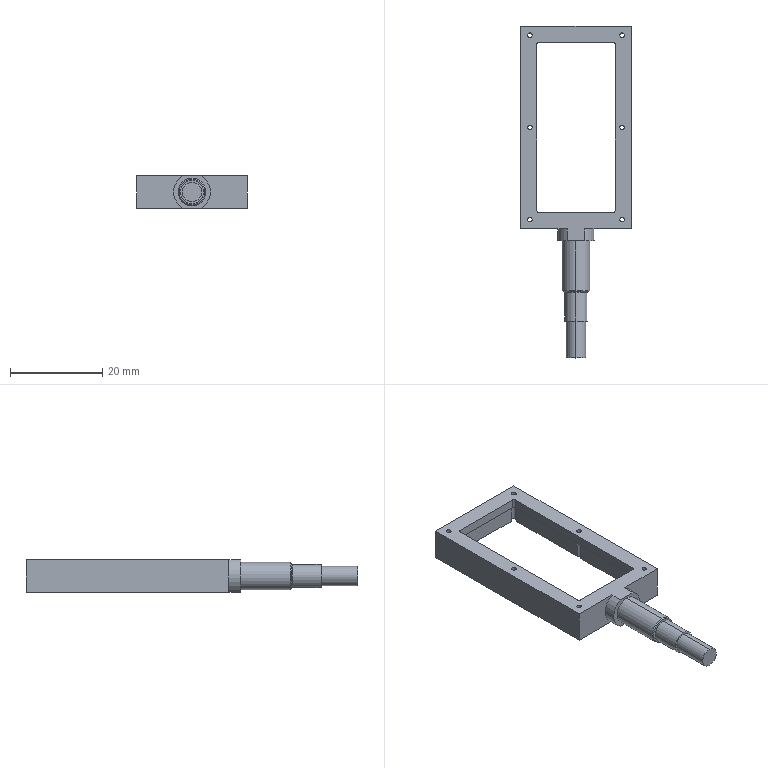NC program | NX | posted with a generic post | part box 24 x 72 x 7 mm
Whole program:
N10 G17 G21 G94 G90
(FLOOR_WALL_COPY , TOOL : D10)
N12 T10 M6
N14 G54
N16 G17 G0 G90 X22. Y11.482 S9500 M3
N18 G43 Z37. H10
N20 Z18.505
N22 G94 G1 Z15.505 F1000.
N24 Y3.482
N26 X0. F2500.
N28 Y-3.482
N30 X44.
N32 Y3.482
N34 X22.
N36 Y11.482
N38 Z18.505
N40 G0 Z37.
N42 Y12.873
N44 Z18.011
N46 G1 Z15.011 F1000.
N48 Y-0.373
N50 X39.5 F2500.
N52 Y0.373
N54 X4.5
N56 Y-0.373
N58 X22.
N60 Y-4.873
N62 X44.
N64 Y4.873
N66 X0.
N68 Y-4.873
N70 X22.
N72 Y-12.873
N74 Z18.011
N76 G0 Z37.
N78 Y-13.907
N80 Z17.516
N82 G1 Z14.516 F1000.
N84 Y-0.907
N86 X39. F2500.
N88 Y0.907
N90 X5.
N92 Y-0.907
N94 X22.
N96 Y-5.907
N98 X44.
N100 Y5.907
N102 X0.
N104 Y-5.907
N106 X22.
N108 Y-13.907
N110 Z17.516
N112 G0 Z37.
N114 Y-14.748
N116 Z17.022
N118 G1 Z14.022 F1000.
N120 Y-1.748
N122 X39. F2500.
N124 Y1.748
N126 X5.
N128 Y-1.748
N130 X22.
N132 Y-6.748
N134 X44.
N136 Y6.748
N138 X0.
N140 Y-6.748
N142 X22.
N144 Y-14.748
N146 Z17.022
N148 G0 Z37.
N150 Y-15.463
N152 Z16.528
N154 G1 Z13.528 F1000.
N156 Y-2.463
N158 X39. F2500.
N160 Y2.463
N162 X5.
N164 Y-2.463
N166 X22.
N168 Y-7.463
N170 X44.
N172 Y7.463
N174 X0.
N176 Y-7.463
N178 X22.
N180 Y-15.463
N182 Z16.528
N184 G0 Z37.
N186 Y-16.085
N188 Z16.033
N190 G1 Z13.033 F1000.
N192 Y-3.085
N194 X39. F2500.
N196 Y3.085
N198 X5.
N200 Y-3.085
N202 X22.
N204 Y-8.085
N206 X44.
N208 Y8.085
N210 X0.
N212 Y-8.085
N214 X22.
N216 Y-16.085
N218 Z16.033
N220 G0 Z37.
N222 Y-16.634
N224 Z15.539
N226 G1 Z12.539 F1000.
N228 Y-3.634
N230 X39. F2500.
N232 Y3.634
N234 X5.
N236 Y-3.634
N238 X22.
N240 Y-8.634
N242 X44.
N244 Y8.634
N246 X0.
N248 Y-8.634
N250 X22.
N252 Y-16.634
N254 Z15.539
N256 G0 Z37.
N258 Y-17.124
N260 Z15.044
N262 G1 Z12.044 F1000.
N264 Y-4.124
N266 X39. F2500.
N268 Y4.124
N270 X5.
N272 Y-4.124
N274 X22.
N276 Y-9.124
N278 X44.
N280 Y9.124
N282 X0.
N284 Y-9.124
N286 X22.
N288 Y-17.124
N290 Z15.044
N292 G0 Z37.
N294 X9.915 Y0.063
N296 Z15.044
N298 G1 X9.5 Z14.933 F1000.
N300 Y-0.063 Z14.899
N302 X22. Z11.55
N304 X34.5 F2500.
N306 Y0.063
N308 X9.5
N310 Y-0.063
N312 X22.
N314 Y-4.563
N316 X39.
N318 Y4.563
N320 X5.
N322 Y-4.563
N324 X22.
N326 Y-9.563
N328 X44.
N330 Y9.563
N332 X0.
N334 Y-9.563
N336 X22.
N338 Y-17.563
N340 Z14.55
N342 G0 Z37.
N344 X9.5 Y0.083
N346 Z14.55
N348 G1 Y-0.458 Z14.405 F1000.
N350 X22. Z11.055
N352 X34.5 F2500.
N354 Y0.458
N356 X9.5
N358 Y-0.458
N360 X22.
N362 Y-4.958
N364 X39.
N366 Y4.958
N368 X5.
N370 Y-4.958
N372 X22.
N374 Y-9.958
N376 X44.
N378 Y9.958
N380 X0.
N382 Y-9.958
N384 X22.
N386 Y-17.958
N388 Z14.055
N390 G0 Z37.
N392 X10.412 Y0.315
N394 Z14.055
N396 G1 X10. Z13.945 F1000.
N398 Y-0.315 Z13.776
N400 X22. Z10.561
N402 X34. F2500.
N404 Y0.315
N406 X10.
N408 Y-0.315
N410 X22.
N412 Y-5.315
N414 X39.
N416 Y5.315
N418 X5.
N420 Y-5.315
N422 X22.
N424 Y-10.315
N426 X44.
N428 Y10.315
N430 X0.
N432 Y-10.315
N434 X22.
N436 Y-18.315
N438 Z13.561
N440 G0 Z37.
N442 X34. Y-0.405
N444 Z13.561
N446 G1 Y0.636 Z13.282 F1000.
N448 X22. Z10.067
N450 X10. F2500.
N452 Y-0.636
N454 X34.
N456 Y0.636
N458 X22.
N460 Y5.636
N462 X5.
N464 Y-5.636
N466 X39.
N468 Y5.636
N470 X22.
N472 Y10.636
N474 X0.
N476 Y-10.636
N478 X44.
N480 Y10.636
N482 X22.
N484 Y18.636
N486 Z13.067
N488 G0 Z37.
N490 X10. Y0.115
N492 Z13.067
N494 G1 Y-0.926 Z12.788 F1000.
N496 X22. Z9.572
N498 X34. F2500.
N500 Y0.926
N502 X10.
N504 Y-0.926
N506 X22.
N508 Y-5.926
N510 X39.
N512 Y5.926
N514 X5.
N516 Y-5.926
N518 X22.
N520 Y-10.926
N522 X44.
N524 Y10.926
N526 X0.
N528 Y-10.926
N530 X22.
N532 Y-18.926
N534 Z12.572
N536 G0 Z37.
N538 X10. Y-0.145
N540 Z12.572
N542 G1 Y-1.187 Z12.293 F1000.
N544 X22. Z9.078
N546 X34. F2500.
N548 Y1.187
N550 X10.
N552 Y-1.187
N554 X22.
N556 Y-6.187
N558 X39.
N560 Y6.187
N562 X5.
N564 Y-6.187
N566 X22.
N568 Y-11.187
N570 X44.
N572 Y11.187
N574 X0.
N576 Y-11.187
N578 X22.
N580 Y-19.187
N582 Z12.078
N584 G0 Z37.
N586 X34. Y0.378
N588 Z12.078
N590 G1 Y1.42 Z11.799 F1000.
N592 X22. Z8.583
N594 X10. F2500.
N596 Y-1.42
N598 X34.
N600 Y1.42
N602 X22.
N604 Y6.42
N606 X5.
N608 Y-6.42
N610 X39.
N612 Y6.42
N614 X22.
N616 Y11.42
N618 X0.
N620 Y-11.42
N622 X44.
N624 Y11.42
N626 X22.
N628 Y19.42
N630 Z11.583
N632 G0 Z37.
N634 X10. Y-0.586
N636 Z11.583
N638 G1 Y-1.627 Z11.304 F1000.
N640 X22. Z8.089
N642 X34. F2500.
N644 Y1.627
N646 X10.
N648 Y-1.627
N650 X22.
N652 Y-6.627
N654 X39.
N656 Y6.627
N658 X5.
N660 Y-6.627
N662 X22.
N664 Y-11.627
N666 X44.
N668 Y11.627
N670 X0.
N672 Y-11.627
N674 X22.
N676 Y-19.627
N678 Z11.089
N680 G0 Z37.
N682 X10. Y-0.769
N684 Z11.089
N686 G1 Y-1.81 Z10.81 F1000.
N688 X22. Z7.594
N690 X34. F2500.
N692 Y1.81
N694 X10.
N696 Y-1.81
N698 X22.
N700 Y-6.81
N702 X39.
N704 Y6.81
N706 X5.
N708 Y-6.81
N710 X22.
N712 Y-11.81
N714 X44.
N716 Y11.81
N718 X0.
N720 Y-11.81
N722 X22.
N724 Y-19.81
N726 Z10.594
N728 G0 Z37.
N730 X10. Y-0.929
N732 Z10.594
N734 G1 Y-1.97 Z10.315 F1000.
N736 X22. Z7.1
N738 X34. F2500.
N740 Y-1.744
N742 G2 X34.153 Y0. R10.
N744 X34. Y1.744 R10.
N746 G1 Y1.97
N748 X10.
N750 Y-1.97
N752 X22.
N754 Y-6.97
N756 X39.
N758 Y-1.744
N760 G2 X39.314 Y0. R5.
N762 X39. Y1.744 R5.
N764 G1 Y6.97
N766 X5.
N768 Y-6.97
N770 X22.
N772 Y-11.97
N774 X44.
N776 Y-1.744
N778 X46.6
N780 Y1.744
N782 X44.
N784 Y11.97
N786 X0.
N788 Y-11.97
N790 X22.
N792 Y-19.97
N794 Z10.1
N796 G0 Z37.
N798 M5
(FLOOR_WALL_1_COPY , TOOL : D10JING)
N800 T11 M6
N802 G54
N804 G17 G0 G90 X52. Y-11.997 S9500 M3
N806 G43 Z37. H11
N808 Z10.
N810 G94 G1 Z7. F1250.
N812 X49.
N814 X-5.
N816 Y-6.998
N818 X49.
N820 X51.6 Y-6.936
N822 Y-1.999
N824 X-5.
N826 Y3.001
N828 X51.6
N830 Y6.936
N832 X49. Y8.
N834 X-5.
N836 X-8.
N838 Z10.
N840 G0 Z37.
N842 M5
(PLANAR_MILL_COPY_COPY_COPY , TOOL : D6A45)
N844 T07 M6
N846 G54
N848 G17 G0 G90 X20.73 Y-6.5 S9500 M3
N850 G43 Z37. H7
N852 Z7.5
N854 G94 G1 Z6. F1250.
N856 X21.134 Y-7.2
N858 G3 X22. Y-7.7 R1.
N860 G1 X39.7
N862 Y7.7
N864 X4.3
N866 Y-7.7
N868 X22.
N870 G3 X22.866 Y-7.2 R1.
N872 G1 X23.27 Y-6.5
N874 Z7.5
N876 G0 Z37.
N878 M5
N880 M2